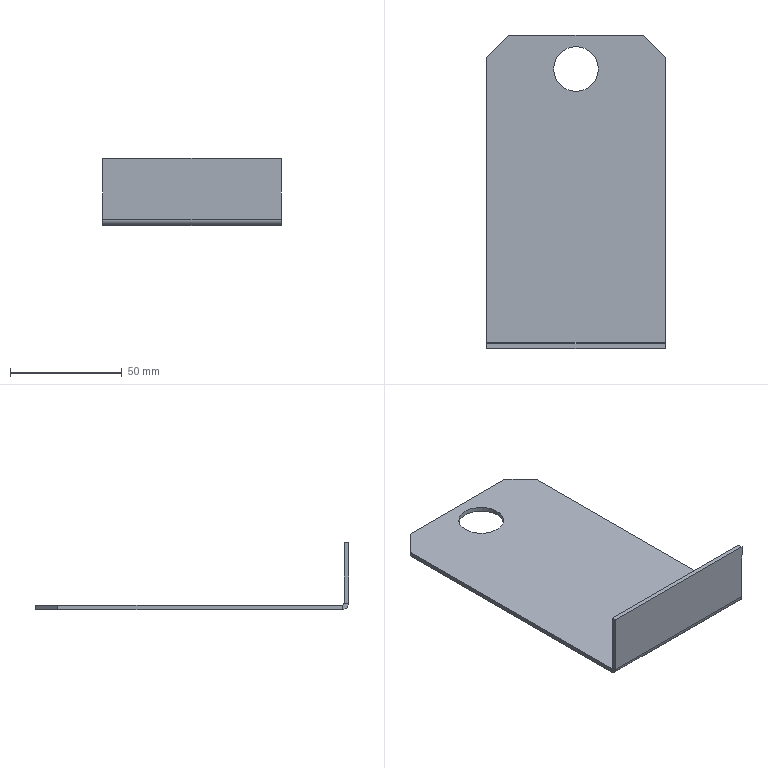Part | SolidWorks | features Chamfer 1, EdgeFlange 1, FlatPattern 1, ICE 1, SMBaseFlange 1, SheetMetal 1 | 1 solid | 18 faces | box 80 x 140 x 30 mm | volume 25932 mm3 | plane 14 | cylinder 4 | commonest cylinder face diameters 20 x2 1.473 x1 5.473 x1
STEP:
#1=CARTESIAN_POINT('',(-10.,55.,-2.));
#2=VERTEX_POINT('',#1);
#3=CARTESIAN_POINT('',(10.,55.,-2.));
#4=VERTEX_POINT('',#3);
#5=CARTESIAN_POINT('',(0.,55.,-2.));
#6=DIRECTION('',(0.,0.,1.));
#7=DIRECTION('',(1.,0.,0.));
#8=AXIS2_PLACEMENT_3D('',#5,#6,#7);
#9=CIRCLE('',#8,10.);
#10=EDGE_CURVE('',#2,#4,#9,.T.);
#11=ORIENTED_EDGE('',*,*,#10,.F.);
#12=CARTESIAN_POINT('',(-10.,55.,0.));
#13=VERTEX_POINT('',#12);
#14=CARTESIAN_POINT('',(-10.,55.,-2.));
#15=DIRECTION('',(0.,0.,1.));
#16=VECTOR('',#15,1000.);
#17=LINE('',#14,#16);
#18=EDGE_CURVE('',#2,#13,#17,.T.);
#19=ORIENTED_EDGE('',*,*,#18,.T.);
#20=CARTESIAN_POINT('',(10.,55.,0.));
#21=VERTEX_POINT('',#20);
#22=CARTESIAN_POINT('',(0.,55.,0.));
#23=DIRECTION('',(0.,0.,1.));
#24=DIRECTION('',(1.,0.,0.));
#25=AXIS2_PLACEMENT_3D('',#22,#23,#24);
#26=CIRCLE('',#25,10.);
#27=EDGE_CURVE('',#13,#21,#26,.T.);
#28=ORIENTED_EDGE('',*,*,#27,.T.);
#29=CARTESIAN_POINT('',(10.,55.,-2.));
#30=DIRECTION('',(0.,0.,1.));
#31=VECTOR('',#30,1000.);
#32=LINE('',#29,#31);
#33=EDGE_CURVE('',#4,#21,#32,.T.);
#34=ORIENTED_EDGE('',*,*,#33,.F.);
#35=EDGE_LOOP('',(#11,#19,#28,#34));
#36=FACE_OUTER_BOUND('',#35,.T.);
#37=CARTESIAN_POINT('',(0.,55.,-2.));
#38=DIRECTION('',(0.,0.,1.));
#39=DIRECTION('',(1.,0.,0.));
#40=AXIS2_PLACEMENT_3D('',#37,#38,#39);
#41=CYLINDRICAL_SURFACE('',#40,10.);
#42=ADVANCED_FACE('',(#36),#41,.F.);
#43=CARTESIAN_POINT('',(40.,-67.263,-2.));
#44=VERTEX_POINT('',#43);
#45=CARTESIAN_POINT('',(40.,60.,-2.));
#46=VERTEX_POINT('',#45);
#47=CARTESIAN_POINT('',(40.,-70.,-2.));
#48=DIRECTION('',(0.,1.,0.));
#49=VECTOR('',#48,1000.);
#50=LINE('',#47,#49);
#51=EDGE_CURVE('',#44,#46,#50,.T.);
#52=ORIENTED_EDGE('',*,*,#51,.T.);
#53=CARTESIAN_POINT('',(40.,60.,0.));
#54=VERTEX_POINT('',#53);
#55=CARTESIAN_POINT('',(40.,60.,-2.));
#56=DIRECTION('',(0.,0.,1.));
#57=VECTOR('',#56,1000.);
#58=LINE('',#55,#57);
#59=EDGE_CURVE('',#46,#54,#58,.T.);
#60=ORIENTED_EDGE('',*,*,#59,.T.);
#61=CARTESIAN_POINT('',(40.,-67.263,0.));
#62=VERTEX_POINT('',#61);
#63=CARTESIAN_POINT('',(40.,-70.,0.));
#64=DIRECTION('',(0.,1.,0.));
#65=VECTOR('',#64,1000.);
#66=LINE('',#63,#65);
#67=EDGE_CURVE('',#62,#54,#66,.T.);
#68=ORIENTED_EDGE('',*,*,#67,.F.);
#69=CARTESIAN_POINT('',(40.,-67.263,0.));
#70=DIRECTION('',(0.,0.,-1.));
#71=VECTOR('',#70,1000.);
#72=LINE('',#69,#71);
#73=EDGE_CURVE('',#62,#44,#72,.T.);
#74=ORIENTED_EDGE('',*,*,#73,.T.);
#75=EDGE_LOOP('',(#52,#60,#68,#74));
#76=FACE_OUTER_BOUND('',#75,.T.);
#77=CARTESIAN_POINT('',(40.,-70.,-2.));
#78=DIRECTION('',(1.,0.,0.));
#79=DIRECTION('',(0.,0.,-1.));
#80=AXIS2_PLACEMENT_3D('',#77,#78,#79);
#81=PLANE('',#80);
#82=ADVANCED_FACE('',(#76),#81,.T.);
#83=CARTESIAN_POINT('',(0.,55.,-2.));
#84=DIRECTION('',(0.,0.,1.));
#85=DIRECTION('',(1.,0.,0.));
#86=AXIS2_PLACEMENT_3D('',#83,#84,#85);
#87=CIRCLE('',#86,10.);
#88=EDGE_CURVE('',#4,#2,#87,.T.);
#89=ORIENTED_EDGE('',*,*,#88,.T.);
#90=ORIENTED_EDGE('',*,*,#10,.T.);
#91=EDGE_LOOP('',(#89,#90));
#92=FACE_BOUND('',#91,.T.);
#93=CARTESIAN_POINT('',(-40.,60.,-2.));
#94=VERTEX_POINT('',#93);
#95=CARTESIAN_POINT('',(-40.,-67.263,-2.));
#96=VERTEX_POINT('',#95);
#97=CARTESIAN_POINT('',(-40.,-70.,-2.));
#98=DIRECTION('',(0.,-1.,0.));
#99=VECTOR('',#98,1000.);
#100=LINE('',#97,#99);
#101=EDGE_CURVE('',#94,#96,#100,.T.);
#102=ORIENTED_EDGE('',*,*,#101,.F.);
#103=CARTESIAN_POINT('',(-30.,70.,-2.));
#104=VERTEX_POINT('',#103);
#105=CARTESIAN_POINT('',(-50.,50.,-2.));
#106=DIRECTION('',(0.7071,0.7071,0.));
#107=VECTOR('',#106,1000.);
#108=LINE('',#105,#107);
#109=EDGE_CURVE('',#94,#104,#108,.T.);
#110=ORIENTED_EDGE('',*,*,#109,.T.);
#111=CARTESIAN_POINT('',(30.,70.,-2.));
#112=VERTEX_POINT('',#111);
#113=CARTESIAN_POINT('',(-40.,70.,-2.));
#114=DIRECTION('',(-1.,0.,0.));
#115=VECTOR('',#114,1000.);
#116=LINE('',#113,#115);
#117=EDGE_CURVE('',#112,#104,#116,.T.);
#118=ORIENTED_EDGE('',*,*,#117,.F.);
#119=CARTESIAN_POINT('',(50.,50.,-2.));
#120=DIRECTION('',(0.7071,-0.7071,0.));
#121=VECTOR('',#120,1000.);
#122=LINE('',#119,#121);
#123=EDGE_CURVE('',#112,#46,#122,.T.);
#124=ORIENTED_EDGE('',*,*,#123,.T.);
#125=ORIENTED_EDGE('',*,*,#51,.F.);
#126=CARTESIAN_POINT('',(40.,-67.263,-2.));
#127=DIRECTION('',(-1.,0.,0.));
#128=VECTOR('',#127,1000.);
#129=LINE('',#126,#128);
#130=EDGE_CURVE('',#44,#96,#129,.T.);
#131=ORIENTED_EDGE('',*,*,#130,.T.);
#132=EDGE_LOOP('',(#102,#110,#118,#124,#125,#131));
#133=FACE_OUTER_BOUND('',#132,.T.);
#134=CARTESIAN_POINT('',(0.,0.,-2.));
#135=DIRECTION('',(0.,0.,-1.));
#136=DIRECTION('',(-1.,0.,0.));
#137=AXIS2_PLACEMENT_3D('',#134,#135,#136);
#138=PLANE('',#137);
#139=ADVANCED_FACE('',(#92,#133),#138,.T.);
#140=CARTESIAN_POINT('',(0.,55.,0.));
#141=DIRECTION('',(0.,0.,1.));
#142=DIRECTION('',(1.,0.,0.));
#143=AXIS2_PLACEMENT_3D('',#140,#141,#142);
#144=CIRCLE('',#143,10.);
#145=EDGE_CURVE('',#21,#13,#144,.T.);
#146=ORIENTED_EDGE('',*,*,#145,.F.);
#147=ORIENTED_EDGE('',*,*,#27,.F.);
#148=EDGE_LOOP('',(#146,#147));
#149=FACE_BOUND('',#148,.T.);
#150=CARTESIAN_POINT('',(30.,70.,0.));
#151=VERTEX_POINT('',#150);
#152=CARTESIAN_POINT('',(-30.,70.,0.));
#153=VERTEX_POINT('',#152);
#154=CARTESIAN_POINT('',(-40.,70.,0.));
#155=DIRECTION('',(-1.,0.,0.));
#156=VECTOR('',#155,1000.);
#157=LINE('',#154,#156);
#158=EDGE_CURVE('',#151,#153,#157,.T.);
#159=ORIENTED_EDGE('',*,*,#158,.T.);
#160=CARTESIAN_POINT('',(-40.,60.,0.));
#161=VERTEX_POINT('',#160);
#162=CARTESIAN_POINT('',(-30.,70.,0.));
#163=DIRECTION('',(-0.7071,-0.7071,0.));
#164=VECTOR('',#163,1000.);
#165=LINE('',#162,#164);
#166=EDGE_CURVE('',#153,#161,#165,.T.);
#167=ORIENTED_EDGE('',*,*,#166,.T.);
#168=CARTESIAN_POINT('',(-40.,-67.263,0.));
#169=VERTEX_POINT('',#168);
#170=CARTESIAN_POINT('',(-40.,-70.,0.));
#171=DIRECTION('',(0.,-1.,0.));
#172=VECTOR('',#171,1000.);
#173=LINE('',#170,#172);
#174=EDGE_CURVE('',#161,#169,#173,.T.);
#175=ORIENTED_EDGE('',*,*,#174,.T.);
#176=CARTESIAN_POINT('',(40.,-67.263,0.));
#177=DIRECTION('',(-1.,0.,0.));
#178=VECTOR('',#177,1000.);
#179=LINE('',#176,#178);
#180=EDGE_CURVE('',#62,#169,#179,.T.);
#181=ORIENTED_EDGE('',*,*,#180,.F.);
#182=ORIENTED_EDGE('',*,*,#67,.T.);
#183=CARTESIAN_POINT('',(40.,60.,0.));
#184=DIRECTION('',(-0.7071,0.7071,0.));
#185=VECTOR('',#184,1000.);
#186=LINE('',#183,#185);
#187=EDGE_CURVE('',#54,#151,#186,.T.);
#188=ORIENTED_EDGE('',*,*,#187,.T.);
#189=EDGE_LOOP('',(#159,#167,#175,#181,#182,#188));
#190=FACE_OUTER_BOUND('',#189,.T.);
#191=CARTESIAN_POINT('',(0.,0.,0.));
#192=DIRECTION('',(0.,0.,-1.));
#193=DIRECTION('',(-1.,0.,0.));
#194=AXIS2_PLACEMENT_3D('',#191,#192,#193);
#195=PLANE('',#194);
#196=ADVANCED_FACE('',(#149,#190),#195,.F.);
#197=ORIENTED_EDGE('',*,*,#174,.F.);
#198=CARTESIAN_POINT('',(-40.,60.,-2.));
#199=DIRECTION('',(0.,0.,-1.));
#200=VECTOR('',#199,1000.);
#201=LINE('',#198,#200);
#202=EDGE_CURVE('',#161,#94,#201,.T.);
#203=ORIENTED_EDGE('',*,*,#202,.T.);
#204=ORIENTED_EDGE('',*,*,#101,.T.);
#205=CARTESIAN_POINT('',(-40.,-67.263,0.));
#206=DIRECTION('',(0.,0.,-1.));
#207=VECTOR('',#206,1000.);
#208=LINE('',#205,#207);
#209=EDGE_CURVE('',#169,#96,#208,.T.);
#210=ORIENTED_EDGE('',*,*,#209,.F.);
#211=EDGE_LOOP('',(#197,#203,#204,#210));
#212=FACE_OUTER_BOUND('',#211,.T.);
#213=CARTESIAN_POINT('',(-40.,-70.,-2.));
#214=DIRECTION('',(-1.,0.,0.));
#215=DIRECTION('',(0.,0.,1.));
#216=AXIS2_PLACEMENT_3D('',#213,#214,#215);
#217=PLANE('',#216);
#218=ADVANCED_FACE('',(#212),#217,.T.);
#219=ORIENTED_EDGE('',*,*,#117,.T.);
#220=CARTESIAN_POINT('',(-30.,70.,-2.));
#221=DIRECTION('',(0.,0.,1.));
#222=VECTOR('',#221,1000.);
#223=LINE('',#220,#222);
#224=EDGE_CURVE('',#104,#153,#223,.T.);
#225=ORIENTED_EDGE('',*,*,#224,.T.);
#226=ORIENTED_EDGE('',*,*,#158,.F.);
#227=CARTESIAN_POINT('',(30.,70.,-2.));
#228=DIRECTION('',(0.,0.,-1.));
#229=VECTOR('',#228,1000.);
#230=LINE('',#227,#229);
#231=EDGE_CURVE('',#151,#112,#230,.T.);
#232=ORIENTED_EDGE('',*,*,#231,.T.);
#233=EDGE_LOOP('',(#219,#225,#226,#232));
#234=FACE_OUTER_BOUND('',#233,.T.);
#235=CARTESIAN_POINT('',(-40.,70.,-2.));
#236=DIRECTION('',(0.,1.,0.));
#237=DIRECTION('',(0.,0.,1.));
#238=AXIS2_PLACEMENT_3D('',#235,#236,#237);
#239=PLANE('',#238);
#240=ADVANCED_FACE('',(#234),#239,.T.);
#241=CARTESIAN_POINT('',(-40.,-68.,0.7366));
#242=VERTEX_POINT('',#241);
#243=CARTESIAN_POINT('',(-40.,-70.,0.7366));
#244=VERTEX_POINT('',#243);
#245=CARTESIAN_POINT('',(-40.,-70.,0.7366));
#246=DIRECTION('',(0.,-1.,0.));
#247=VECTOR('',#246,1000.);
#248=LINE('',#245,#247);
#249=EDGE_CURVE('',#242,#244,#248,.T.);
#250=ORIENTED_EDGE('',*,*,#249,.F.);
#251=CARTESIAN_POINT('',(-40.,-67.263,0.7366));
#252=DIRECTION('',(-1.,0.,0.));
#253=DIRECTION('',(0.,0.,-1.));
#254=AXIS2_PLACEMENT_3D('',#251,#252,#253);
#255=CIRCLE('',#254,0.7366);
#256=EDGE_CURVE('',#169,#242,#255,.T.);
#257=ORIENTED_EDGE('',*,*,#256,.F.);
#258=ORIENTED_EDGE('',*,*,#209,.T.);
#259=CARTESIAN_POINT('',(-40.,-67.263,0.7366));
#260=DIRECTION('',(-1.,0.,0.));
#261=DIRECTION('',(0.,0.,-1.));
#262=AXIS2_PLACEMENT_3D('',#259,#260,#261);
#263=CIRCLE('',#262,2.737);
#264=EDGE_CURVE('',#96,#244,#263,.T.);
#265=ORIENTED_EDGE('',*,*,#264,.T.);
#266=EDGE_LOOP('',(#250,#257,#258,#265));
#267=FACE_OUTER_BOUND('',#266,.T.);
#268=CARTESIAN_POINT('',(-40.,-67.263,0.7366));
#269=DIRECTION('',(-1.,0.,0.));
#270=DIRECTION('',(0.,0.,1.));
#271=AXIS2_PLACEMENT_3D('',#268,#269,#270);
#272=PLANE('',#271);
#273=ADVANCED_FACE('',(#267),#272,.T.);
#274=CARTESIAN_POINT('',(40.,-68.,0.7366));
#275=VERTEX_POINT('',#274);
#276=CARTESIAN_POINT('',(40.,-67.263,0.7366));
#277=DIRECTION('',(1.,0.,0.));
#278=DIRECTION('',(0.,0.,-1.));
#279=AXIS2_PLACEMENT_3D('',#276,#277,#278);
#280=CIRCLE('',#279,0.7366);
#281=EDGE_CURVE('',#275,#62,#280,.T.);
#282=ORIENTED_EDGE('',*,*,#281,.F.);
#283=CARTESIAN_POINT('',(40.,-70.,0.7366));
#284=VERTEX_POINT('',#283);
#285=CARTESIAN_POINT('',(40.,-68.,0.7366));
#286=DIRECTION('',(0.,-1.,0.));
#287=VECTOR('',#286,1000.);
#288=LINE('',#285,#287);
#289=EDGE_CURVE('',#275,#284,#288,.T.);
#290=ORIENTED_EDGE('',*,*,#289,.T.);
#291=CARTESIAN_POINT('',(40.,-67.263,0.7366));
#292=DIRECTION('',(1.,0.,0.));
#293=DIRECTION('',(0.,0.,-1.));
#294=AXIS2_PLACEMENT_3D('',#291,#292,#293);
#295=CIRCLE('',#294,2.737);
#296=EDGE_CURVE('',#284,#44,#295,.T.);
#297=ORIENTED_EDGE('',*,*,#296,.T.);
#298=ORIENTED_EDGE('',*,*,#73,.F.);
#299=EDGE_LOOP('',(#282,#290,#297,#298));
#300=FACE_OUTER_BOUND('',#299,.T.);
#301=CARTESIAN_POINT('',(40.,-67.263,0.7366));
#302=DIRECTION('',(-1.,0.,0.));
#303=DIRECTION('',(0.,0.,1.));
#304=AXIS2_PLACEMENT_3D('',#301,#302,#303);
#305=PLANE('',#304);
#306=ADVANCED_FACE('',(#300),#305,.F.);
#307=ORIENTED_EDGE('',*,*,#130,.F.);
#308=ORIENTED_EDGE('',*,*,#296,.F.);
#309=CARTESIAN_POINT('',(-40.,-70.,0.7366));
#310=DIRECTION('',(-1.,0.,0.));
#311=VECTOR('',#310,1000.);
#312=LINE('',#309,#311);
#313=EDGE_CURVE('',#284,#244,#312,.T.);
#314=ORIENTED_EDGE('',*,*,#313,.T.);
#315=ORIENTED_EDGE('',*,*,#264,.F.);
#316=EDGE_LOOP('',(#307,#308,#314,#315));
#317=FACE_OUTER_BOUND('',#316,.T.);
#318=CARTESIAN_POINT('',(40.,-67.263,0.7366));
#319=DIRECTION('',(1.,0.,0.));
#320=DIRECTION('',(0.,-1.,0.));
#321=AXIS2_PLACEMENT_3D('',#318,#319,#320);
#322=CYLINDRICAL_SURFACE('',#321,2.737);
#323=ADVANCED_FACE('',(#317),#322,.T.);
#324=ORIENTED_EDGE('',*,*,#180,.T.);
#325=ORIENTED_EDGE('',*,*,#256,.T.);
#326=CARTESIAN_POINT('',(-40.,-68.,0.7366));
#327=DIRECTION('',(1.,0.,0.));
#328=VECTOR('',#327,1000.);
#329=LINE('',#326,#328);
#330=EDGE_CURVE('',#242,#275,#329,.T.);
#331=ORIENTED_EDGE('',*,*,#330,.T.);
#332=ORIENTED_EDGE('',*,*,#281,.T.);
#333=EDGE_LOOP('',(#324,#325,#331,#332));
#334=FACE_OUTER_BOUND('',#333,.T.);
#335=CARTESIAN_POINT('',(40.,-67.263,0.7366));
#336=DIRECTION('',(1.,0.,0.));
#337=DIRECTION('',(0.,-1.,0.));
#338=AXIS2_PLACEMENT_3D('',#335,#336,#337);
#339=CYLINDRICAL_SURFACE('',#338,0.7366);
#340=ADVANCED_FACE('',(#334),#339,.F.);
#341=ORIENTED_EDGE('',*,*,#249,.T.);
#342=CARTESIAN_POINT('',(-40.,-70.,28.));
#343=VERTEX_POINT('',#342);
#344=CARTESIAN_POINT('',(-40.,-70.,0.));
#345=DIRECTION('',(0.,0.,-1.));
#346=VECTOR('',#345,1000.);
#347=LINE('',#344,#346);
#348=EDGE_CURVE('',#343,#244,#347,.T.);
#349=ORIENTED_EDGE('',*,*,#348,.F.);
#350=CARTESIAN_POINT('',(-40.,-68.,28.));
#351=VERTEX_POINT('',#350);
#352=CARTESIAN_POINT('',(-40.,-70.,28.));
#353=DIRECTION('',(0.,1.,0.));
#354=VECTOR('',#353,1000.);
#355=LINE('',#352,#354);
#356=EDGE_CURVE('',#343,#351,#355,.T.);
#357=ORIENTED_EDGE('',*,*,#356,.T.);
#358=CARTESIAN_POINT('',(-40.,-68.,0.));
#359=DIRECTION('',(0.,0.,-1.));
#360=VECTOR('',#359,1000.);
#361=LINE('',#358,#360);
#362=EDGE_CURVE('',#351,#242,#361,.T.);
#363=ORIENTED_EDGE('',*,*,#362,.T.);
#364=EDGE_LOOP('',(#341,#349,#357,#363));
#365=FACE_OUTER_BOUND('',#364,.T.);
#366=CARTESIAN_POINT('',(-40.,-70.,0.));
#367=DIRECTION('',(1.,0.,0.));
#368=DIRECTION('',(0.,0.,-1.));
#369=AXIS2_PLACEMENT_3D('',#366,#367,#368);
#370=PLANE('',#369);
#371=ADVANCED_FACE('',(#365),#370,.F.);
#372=ORIENTED_EDGE('',*,*,#289,.F.);
#373=CARTESIAN_POINT('',(40.,-68.,28.));
#374=VERTEX_POINT('',#373);
#375=CARTESIAN_POINT('',(40.,-68.,28.));
#376=DIRECTION('',(0.,0.,1.));
#377=VECTOR('',#376,1000.);
#378=LINE('',#375,#377);
#379=EDGE_CURVE('',#275,#374,#378,.T.);
#380=ORIENTED_EDGE('',*,*,#379,.T.);
#381=CARTESIAN_POINT('',(40.,-70.,28.));
#382=VERTEX_POINT('',#381);
#383=CARTESIAN_POINT('',(40.,-70.,28.));
#384=DIRECTION('',(0.,1.,0.));
#385=VECTOR('',#384,1000.);
#386=LINE('',#383,#385);
#387=EDGE_CURVE('',#382,#374,#386,.T.);
#388=ORIENTED_EDGE('',*,*,#387,.F.);
#389=CARTESIAN_POINT('',(40.,-70.,0.));
#390=DIRECTION('',(0.,0.,1.));
#391=VECTOR('',#390,1000.);
#392=LINE('',#389,#391);
#393=EDGE_CURVE('',#284,#382,#392,.T.);
#394=ORIENTED_EDGE('',*,*,#393,.F.);
#395=EDGE_LOOP('',(#372,#380,#388,#394));
#396=FACE_OUTER_BOUND('',#395,.T.);
#397=CARTESIAN_POINT('',(40.,-70.,28.));
#398=DIRECTION('',(-1.,0.,0.));
#399=DIRECTION('',(0.,0.,1.));
#400=AXIS2_PLACEMENT_3D('',#397,#398,#399);
#401=PLANE('',#400);
#402=ADVANCED_FACE('',(#396),#401,.F.);
#403=ORIENTED_EDGE('',*,*,#313,.F.);
#404=ORIENTED_EDGE('',*,*,#393,.T.);
#405=CARTESIAN_POINT('',(0.,-70.,28.));
#406=DIRECTION('',(-1.,0.,0.));
#407=VECTOR('',#406,1000.);
#408=LINE('',#405,#407);
#409=EDGE_CURVE('',#382,#343,#408,.T.);
#410=ORIENTED_EDGE('',*,*,#409,.T.);
#411=ORIENTED_EDGE('',*,*,#348,.T.);
#412=EDGE_LOOP('',(#403,#404,#410,#411));
#413=FACE_OUTER_BOUND('',#412,.T.);
#414=CARTESIAN_POINT('',(0.,-70.,0.));
#415=DIRECTION('',(0.,1.,0.));
#416=DIRECTION('',(0.,0.,1.));
#417=AXIS2_PLACEMENT_3D('',#414,#415,#416);
#418=PLANE('',#417);
#419=ADVANCED_FACE('',(#413),#418,.F.);
#420=ORIENTED_EDGE('',*,*,#379,.F.);
#421=ORIENTED_EDGE('',*,*,#330,.F.);
#422=ORIENTED_EDGE('',*,*,#362,.F.);
#423=CARTESIAN_POINT('',(-40.,-68.,28.));
#424=DIRECTION('',(-1.,0.,0.));
#425=VECTOR('',#424,1000.);
#426=LINE('',#423,#425);
#427=EDGE_CURVE('',#374,#351,#426,.T.);
#428=ORIENTED_EDGE('',*,*,#427,.F.);
#429=EDGE_LOOP('',(#420,#421,#422,#428));
#430=FACE_OUTER_BOUND('',#429,.T.);
#431=CARTESIAN_POINT('',(0.,-68.,0.));
#432=DIRECTION('',(0.,1.,0.));
#433=DIRECTION('',(0.,0.,1.));
#434=AXIS2_PLACEMENT_3D('',#431,#432,#433);
#435=PLANE('',#434);
#436=ADVANCED_FACE('',(#430),#435,.T.);
#437=ORIENTED_EDGE('',*,*,#427,.T.);
#438=ORIENTED_EDGE('',*,*,#356,.F.);
#439=ORIENTED_EDGE('',*,*,#409,.F.);
#440=ORIENTED_EDGE('',*,*,#387,.T.);
#441=EDGE_LOOP('',(#437,#438,#439,#440));
#442=FACE_OUTER_BOUND('',#441,.T.);
#443=CARTESIAN_POINT('',(-40.,-70.,28.));
#444=DIRECTION('',(0.,0.,-1.));
#445=DIRECTION('',(0.,1.,0.));
#446=AXIS2_PLACEMENT_3D('',#443,#444,#445);
#447=PLANE('',#446);
#448=ADVANCED_FACE('',(#442),#447,.F.);
#449=ORIENTED_EDGE('',*,*,#18,.F.);
#450=ORIENTED_EDGE('',*,*,#88,.F.);
#451=ORIENTED_EDGE('',*,*,#33,.T.);
#452=ORIENTED_EDGE('',*,*,#145,.T.);
#453=EDGE_LOOP('',(#449,#450,#451,#452));
#454=FACE_OUTER_BOUND('',#453,.T.);
#455=CARTESIAN_POINT('',(0.,55.,-2.));
#456=DIRECTION('',(0.,0.,1.));
#457=DIRECTION('',(1.,0.,0.));
#458=AXIS2_PLACEMENT_3D('',#455,#456,#457);
#459=CYLINDRICAL_SURFACE('',#458,10.);
#460=ADVANCED_FACE('',(#454),#459,.F.);
#461=ORIENTED_EDGE('',*,*,#109,.F.);
#462=ORIENTED_EDGE('',*,*,#202,.F.);
#463=ORIENTED_EDGE('',*,*,#166,.F.);
#464=ORIENTED_EDGE('',*,*,#224,.F.);
#465=EDGE_LOOP('',(#461,#462,#463,#464));
#466=FACE_OUTER_BOUND('',#465,.T.);
#467=CARTESIAN_POINT('',(-30.,70.,-2.));
#468=DIRECTION('',(0.7071,-0.7071,0.));
#469=DIRECTION('',(0.,0.,1.));
#470=AXIS2_PLACEMENT_3D('',#467,#468,#469);
#471=PLANE('',#470);
#472=ADVANCED_FACE('',(#466),#471,.F.);
#473=ORIENTED_EDGE('',*,*,#123,.F.);
#474=ORIENTED_EDGE('',*,*,#231,.F.);
#475=ORIENTED_EDGE('',*,*,#187,.F.);
#476=ORIENTED_EDGE('',*,*,#59,.F.);
#477=EDGE_LOOP('',(#473,#474,#475,#476));
#478=FACE_OUTER_BOUND('',#477,.T.);
#479=CARTESIAN_POINT('',(40.,60.,-2.));
#480=DIRECTION('',(-0.7071,-0.7071,0.));
#481=DIRECTION('',(0.,0.,1.));
#482=AXIS2_PLACEMENT_3D('',#479,#480,#481);
#483=PLANE('',#482);
#484=ADVANCED_FACE('',(#478),#483,.F.);
#485=CLOSED_SHELL('',(#42,#82,#139,#196,#218,#240,#273,#306,#323,#340,#371,#402,#419,#436,#448,#460,#472,#484));
#486=MANIFOLD_SOLID_BREP('',#485);
#487=CARTESIAN_POINT('',(0.,0.,0.));
#488=DIRECTION('',(0.,0.,1.));
#489=DIRECTION('',(1.,0.,0.));
#490=AXIS2_PLACEMENT_3D('',#487,#488,#489);
#491=(LENGTH_UNIT()NAMED_UNIT(*)SI_UNIT(.MILLI.,.METRE.));
#492=UNCERTAINTY_MEASURE_WITH_UNIT(LENGTH_MEASURE(0.00001),#491,'','');
#493=(NAMED_UNIT(*)PLANE_ANGLE_UNIT()SI_UNIT($,.RADIAN.));
#494=(NAMED_UNIT(*)SI_UNIT($,.STERADIAN.)SOLID_ANGLE_UNIT());
#495=(GEOMETRIC_REPRESENTATION_CONTEXT(3)GLOBAL_UNCERTAINTY_ASSIGNED_CONTEXT((#492))GLOBAL_UNIT_ASSIGNED_CONTEXT((#491,#493,#494))REPRESENTATION_CONTEXT('',''));
#496=ADVANCED_BREP_SHAPE_REPRESENTATION('',(#486,#490),#495);